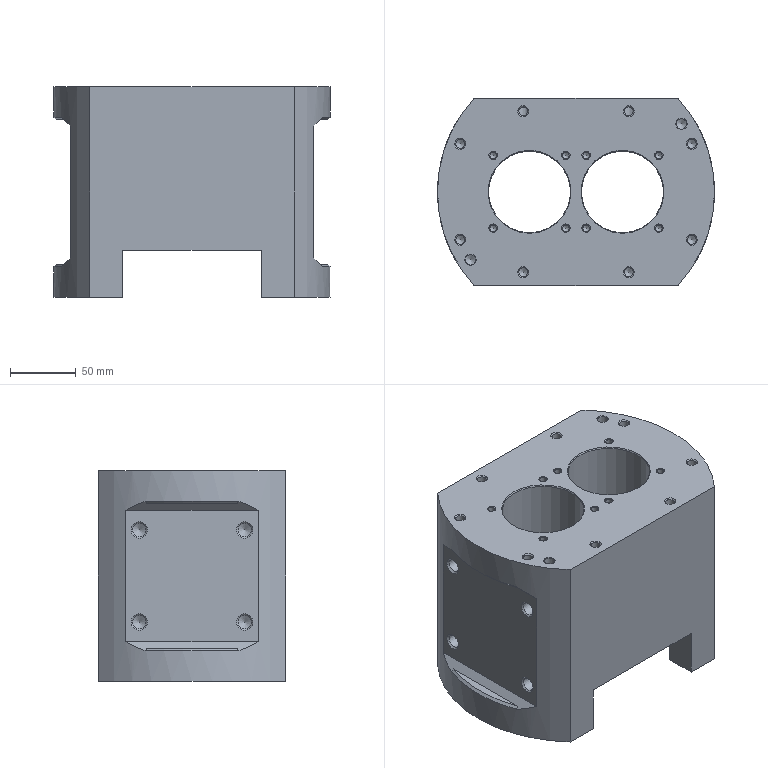NC program | NX | posted with a generic post | part box 210 x 142 x 160 mm
Lines 470 to 2090 of 4789, first 1533 of 1619 lines:
(ZLEVEL_PROFILE_COPY , TOOL : D10)
N932 T10 M6
N934 G54
N936 G17 G0 G90 X-54.432 Y32.868 B0. C0. S3500 M3
N938 G43 Z30. H10
N940 Z2.859
N942 G94 G1 Z-0.141 F1000.
N944 X-55.511 Y31.778
N946 G3 X-55.764 Y30.811 R1.
N948 G2 X-51.879 Y8.915 R121.943 F2200.
N950 X-53.503 Y-20.951 R111.959
N952 X-55.764 Y-30.811 R130.983
N954 G1 X-55.765 Y-30.984 Z-0.189
N956 X-55.768 Y-31.156 Z-0.236
N958 X-55.772 Y-31.328 Z-0.283
N960 G3 X-53.364 Y-20.951 R129.193
N962 G1 X-53.281 Y-20.505
N964 G3 X-51.988 Y11.59 R111.539
N966 X-55.772 Y31.328 R123.16
N968 G1 X-55.773 Y31.499 Z-0.33
N970 X-55.776 Y31.67 Z-0.377
N972 X-55.78 Y31.84 Z-0.424
N974 G2 X-52.279 Y15.115 R123.455
N976 X-52.684 Y-17.865 R110.827
N978 X-55.78 Y-31.84 R127.123
N980 G1 X-55.781 Y-32.011 Z-0.471
N982 X-55.783 Y-32.182 Z-0.519
N984 X-55.787 Y-32.352 Z-0.566
N986 G3 X-53.085 Y-20.951 R129.934
N988 X-51.753 Y12.035 R111.53
N990 X-55.788 Y32.352 R123.802
N992 G1 Y32.521 Z-0.613
N994 X-55.79 Y32.69 Z-0.66
N996 X-55.795 Y32.858 Z-0.707
N998 G2 X-51.882 Y14.264 R125.341
N1000 G1 X-51.666 Y12.481
N1002 G2 X-52.946 Y-20.951 R111.309
N1004 G1 X-53.031 Y-21.396
N1006 X-53.121 Y-21.842
N1008 G2 X-55.795 Y-32.858 R131.028
N1010 G1 X-55.797 Y-33.025 Z-0.754
N1012 X-55.8 Y-33.19 Z-0.801
N1014 X-55.804 Y-33.356 Z-0.849
N1016 G3 X-52.982 Y-21.842 R131.167
N1018 G1 X-52.893 Y-21.396
N1020 X-52.807 Y-20.951
N1022 G3 X-51.525 Y12.481 R111.179
N1024 G1 X-51.741 Y14.264
N1026 G3 X-55.804 Y33.356 R125.503
N1028 G1 X-55.807 Y33.521 Z-0.896
N1030 X-55.81 Y33.686 Z-0.943
N1032 X-55.814 Y33.851 Z-0.99
N1034 G2 X-51.657 Y14.71 R127.282
N1036 X-52.754 Y-21.396 R111.065
N1038 G1 X-52.843 Y-21.842
N1040 G2 X-55.814 Y-33.851 R132.662
N1042 G1 X-55.818 Y-34.012 Z-1.037
N1044 X-55.822 Y-34.173 Z-1.084
N1046 X-55.826 Y-34.334 Z-1.131
N1048 G3 X-52.705 Y-21.842 R131.086
N1050 G1 X-52.615 Y-21.396
N1052 G3 X-51.517 Y14.71 R110.891
N1054 X-55.826 Y34.334 R126.821
N1056 G1 X-55.831 Y34.495 Z-1.179
N1058 X-55.835 Y34.656 Z-1.226
N1060 X-55.841 Y34.816 Z-1.273
N1062 G2 X-51.377 Y14.71 R126.454
N1064 X-52.476 Y-21.396 R110.775
N1066 G1 X-52.566 Y-21.842
N1068 G2 X-55.841 Y-34.816 R130.126
N1070 G1 X-55.843 Y-34.978 Z-1.32
N1072 X-55.848 Y-35.139 Z-1.367
N1074 X-55.856 Y-35.298 Z-1.414
N1076 G3 X-52.427 Y-21.842 R130.376
N1078 G1 X-52.337 Y-21.396
N1080 G3 X-51.237 Y14.71 R110.658
N1082 X-55.856 Y35.298 R126.434
N1084 G1 Y35.459 Z-1.461
N1086 X-55.86 Y35.62 Z-1.508
N1088 X-55.871 Y35.778 Z-1.556
N1090 G2 X-51.097 Y14.71 R126.474
N1092 X-52.027 Y-20.505 R110.646
N1094 G1 X-52.111 Y-20.951
N1096 X-52.198 Y-21.396
N1098 X-52.288 Y-21.842
N1100 G2 X-55.871 Y-35.778 R131.039
N1102 G1 X-55.872 Y-35.939 Z-1.603
N1104 X-55.877 Y-36.098 Z-1.65
N1106 X-55.888 Y-36.255 Z-1.697
N1108 G3 X-51.496 Y-18.276 R129.399
N1110 X-51.349 Y17.385 R110.064
N1112 X-55.888 Y36.254 R129.287
N1114 G1 X-55.875 Y36.442 Z-1.768
N1116 X-55.868 Y36.628 Z-1.839
N1118 G2 X-51.281 Y17.83 R130.392
N1120 X-49.981 Y5.892 R114.798
N1122 X-49.9 Y3.02 R51.132
N1124 G1 Y-2.81
N1126 G2 X-50.037 Y-6.912 R61.409
N1128 X-53.454 Y-28.219 R117.255
N1130 G1 X-53.566 Y-28.655
N1132 G2 X-55.868 Y-36.629 R138.665
N1134 G1 X-55.801 Y-36.638 Z-1.909
N1136 X-55.709 Y-36.651 Z-1.98
N1138 X-55.636 Y-36.329
N1140 G3 X-53.174 Y-27.657 R143.814
N1142 X-50.01 Y-8.459 R118.727
N1144 X-49.9 Y-6.104 R34.261
N1146 G1 Y6.101
N1148 G3 X-50.011 Y8.469 R34.228
N1150 X-51.069 Y17.385 R117.375
N1152 X-55.289 Y35.215 R128.669
N1154 G1 X-55.653 Y36.391
N1156 G2 X-55.711 Y36.653 R1.62
N1158 G1 X-55.607 Y36.717 Z-2.051
N1160 X-55.524 Y36.779 Z-2.122
N1162 G3 X-55.381 Y35.942 R3.116
N1164 G1 X-55.292 Y35.661
N1166 G2 X-51.003 Y17.83 R129.054
N1168 X-49.949 Y9.361 R112.033
N1170 X-49.9 Y8.147 R16.61
N1172 G1 Y-8.249
N1174 G2 X-49.949 Y-9.361 R12.702
N1176 X-53.488 Y-29.42 R117.251
N1178 X-55.386 Y-35.966 R152.214
N1180 G3 X-55.513 Y-36.782 R2.768
N1182 G1 X-55.435 Y-36.945 Z-2.193
N1184 X-55.364 Y-37.108 Z-2.264
N1186 G2 X-55.295 Y-36.106 R10.195
N1188 G1 X-54.216 Y-32.54
N1190 X-54.089 Y-32.095
N1192 G3 X-50.017 Y-11.59 R120.931
N1194 X-49.9 Y-9.783 R18.135
N1196 G1 Y9.777
N1198 G3 X-50.017 Y11.59 R18.122
N1200 X-50.789 Y17.385 R128.233
N1202 X-55.298 Y36.106 R129.171
N1204 G2 X-55.365 Y37.107 R18.316
N1206 G1 X-55.283 Y37.269 Z-2.335
N1208 X-55.209 Y37.43 Z-2.407
N1210 X-55.183 Y36.329
N1212 X-55.162 Y36.106
N1214 G2 X-50.648 Y17.385 R129.227
N1216 X-49.966 Y12.339 R92.528
N1218 X-49.9 Y11.174 R11.539
N1220 G1 Y-11.172
N1222 G2 X-49.982 Y-12.481 R11.538
N1224 G1 X-50.015 Y-12.761
N1226 G2 X-53.142 Y-29.144 R118.996
N1228 X-55.159 Y-36.106 R155.69
N1230 G1 X-55.187 Y-36.329
N1232 X-55.208 Y-37.431
N1234 X-55.132 Y-37.584 Z-2.478
N1236 X-55.068 Y-37.738 Z-2.549
N1238 X-55.044 Y-36.329
N1240 X-55.023 Y-36.106
N1242 X-53.945 Y-32.54
N1244 X-53.815 Y-32.095
N1246 G3 X-50.053 Y-14.264 R122.421
N1248 G1 X-49.966 Y-13.53
N1250 G3 X-49.9 Y-12.411 R12.183
N1252 G1 Y12.41
N1254 G3 X-50.025 Y14.055 R14.641
N1256 X-51.051 Y20.505 R128.491
N1258 X-55.027 Y36.106 R132.287
N1260 G1 X-55.066 Y37.739
N1262 X-54.985 Y37.895 Z-2.62
N1264 X-54.918 Y38.051 Z-2.691
N1266 X-54.912 Y37.889
N1268 X-54.893 Y36.329
N1270 X-54.888 Y36.106
N1272 G2 X-50.911 Y20.505 R132.992
N1274 X-49.979 Y14.737 R101.49
N1276 X-49.9 Y13.534 R9.164
N1278 G1 Y-13.531
N1280 G2 X-49.976 Y-14.71 R9.171
N1282 X-53.809 Y-32.54 R121.679
N1284 G1 X-53.939 Y-32.986
N1286 X-54.887 Y-36.106
N1288 X-54.902 Y-36.329
N1290 X-54.913 Y-37.889
N1292 X-54.918 Y-38.05
N1294 X-54.844 Y-38.217 Z-2.762
N1296 X-54.775 Y-38.384 Z-2.833
N1298 X-54.773 Y-38.335
N1300 X-54.761 Y-36.329
N1302 X-54.749 Y-36.106
N1304 G3 X-53.042 Y-30.312 R181.888
N1306 X-49.985 Y-15.743 R119.356
N1308 X-49.9 Y-14.569 R8.156
N1310 G1 Y14.569
N1312 G3 X-49.985 Y15.748 R8.172
N1314 X-53.785 Y32.904 R120.132
N1316 G1 X-54.745 Y36.106
N1318 X-54.749 Y36.329
N1320 X-54.775 Y38.385
N1322 X-54.703 Y38.577 Z-2.904
N1324 X-54.633 Y38.768 Z-2.974
N1326 X-54.631 Y38.335
N1328 X-54.602 Y36.106
N1330 X-54.504 Y35.74
N1332 X-53.801 Y33.432
N1334 G2 X-50.089 Y17.385 R124.616
N1336 G1 X-50.019 Y16.939
N1338 G2 X-49.9 Y15.521 R9.442
N1340 G1 Y-15.524
N1342 G2 X-50.019 Y-16.939 R9.447
N1344 X-53.668 Y-32.986 R123.555
N1346 G1 X-53.801 Y-33.432
N1348 X-54.48 Y-35.661
N1350 X-54.611 Y-36.106
N1352 X-54.62 Y-36.329
N1354 X-54.632 Y-38.335
N1356 X-54.633 Y-38.768
N1358 X-54.562 Y-38.96 Z-3.045
N1360 X-54.492 Y-39.151 Z-3.116
N1362 X-54.491 Y-38.781
N1364 X-54.478 Y-36.329
N1366 X-54.473 Y-36.106
N1368 X-54.346 Y-35.661
N1370 X-53.666 Y-33.432
N1372 G3 X-50.027 Y-17.83 R123.17
N1374 X-49.9 Y-16.424 R8.031
N1376 G1 Y16.425
N1378 G3 X-50.007 Y17.714 R8.031
N1380 X-53.787 Y33.832 R123.645
N1382 G1 X-54.359 Y35.702
N1384 G2 X-54.459 Y36.106 R3.701
N1386 G1 X-54.492 Y39.152
N1388 X-54.421 Y39.339 Z-3.187
N1390 X-54.355 Y39.526 Z-3.257
N1392 X-54.315 Y36.106
N1394 G3 X-54.19 Y35.584 R4.242
N1396 G1 X-53.693 Y33.971
N1398 G2 X-50.03 Y18.661 R123.357
N1400 X-49.9 Y17.281 R8.995
N1402 G1 Y-17.278
N1404 G2 X-50.041 Y-18.722 R8.99
N1406 X-53.531 Y-33.432 R122.752
N1408 G1 X-54.211 Y-35.661
N1410 X-54.329 Y-36.106
N1412 X-54.335 Y-36.329
N1414 X-54.355 Y-39.526
N1416 X-54.28 Y-39.711 Z-3.328
N1418 X-54.214 Y-39.897 Z-3.399
N1420 X-54.197 Y-36.552
N1422 X-54.186 Y-36.106
N1424 G2 X-54.039 Y-35.54 R6.811
N1426 G1 X-53.621 Y-34.167
N1428 G3 X-50.054 Y-19.613 R124.955
N1430 X-49.9 Y-18.069 R8.702
N1432 G1 Y18.072
N1434 G3 X-50.013 Y19.375 R7.582
N1436 G1 X-50.132 Y20.059
N1438 G3 X-53.561 Y33.978 R126.794
N1440 G1 X-54.059 Y35.599
N1442 G2 X-54.171 Y36.106 R3.233
N1444 X-54.214 Y39.897 R175.513
N1446 G1 X-54.139 Y40.082 Z-3.469
N1448 X-54.071 Y40.268 Z-3.54
N1450 G3 X-54.01 Y35.884 R87.494
N1452 G2 X-50.043 Y20.308 R133.117
N1454 X-49.9 Y18.872 R7.449
N1456 G1 Y-18.868
N1458 G2 X-50.045 Y-20.342 R8.156
N1460 X-53.807 Y-35.215 R129.914
N1462 G1 X-54.01 Y-35.884
N1464 X-54.043 Y-36.106
N1466 X-54.056 Y-36.552
N1468 X-54.071 Y-40.268
N1470 X-53.997 Y-40.452 Z-3.611
N1472 X-53.93 Y-40.636 Z-3.682
N1474 X-53.918 Y-36.998
N1476 X-53.898 Y-36.045
N1478 X-53.899 Y-35.947
N1480 X-53.868 Y-35.854
N1482 X-53.673 Y-35.215
N1484 G3 X-50.031 Y-20.951 R126.56
N1486 X-49.9 Y-19.613 R8.173
N1488 G1 Y19.613
N1490 G3 X-50.031 Y20.951 R8.172
N1492 G1 X-50.478 Y23.179
N1494 G3 X-53.874 Y35.884 R137.422
N1496 G2 X-53.93 Y40.636 R126.824
N1498 G1 X-53.856 Y40.817 Z-3.752
N1500 X-53.786 Y40.997 Z-3.823
N1502 G3 X-53.738 Y35.884 R149.927
N1504 G2 X-51.271 Y27.191 R149.04
N1506 X-50.039 Y21.691 R108.525
N1508 X-49.9 Y20.31 R7.73
N1510 G1 Y-20.31
N1512 G2 X-50.04 Y-21.693 R7.73
N1514 G1 X-50.157 Y-22.288
N1516 G2 X-53.701 Y-35.742 R131.324
N1518 G3 X-53.755 Y-36.065 R1.144
N1520 G1 X-53.777 Y-36.998
N1522 X-53.786 Y-40.997
N1524 X-53.715 Y-41.175 Z-3.894
N1526 X-53.647 Y-41.353 Z-3.964
N1528 X-53.627 Y-36.552
N1530 X-53.606 Y-35.884
N1532 X-52.927 Y-33.664
N1534 G3 X-50.082 Y-22.614 R127.066
N1536 X-49.9 Y-21.023 R8.589
N1538 G1 Y21.024
N1540 G3 X-50.107 Y22.734 R8.344
N1542 X-53.602 Y35.884 R137.68
N1544 G2 X-53.647 Y41.353 R180.835
N1546 G1 X-53.573 Y41.531 Z-4.035
N1548 X-53.507 Y41.709 Z-4.106
N1550 X-53.488 Y36.998
N1552 X-53.464 Y35.884
N1554 G2 X-51.982 Y30.899 R200.497
N1556 X-50.045 Y23.08 R121.054
N1558 X-49.9 Y21.692 R6.607
N1560 G1 Y-21.693
N1562 G2 X-50.066 Y-23.179 R6.607
N1564 X-53.271 Y-35.215 R128.592
N1566 G1 X-53.465 Y-35.884
N1568 X-53.494 Y-36.998
N1570 X-53.507 Y-41.709
N1572 X-53.432 Y-41.886 Z-4.177
N1574 X-53.365 Y-42.062 Z-4.247
N1576 X-53.352 Y-36.998
N1578 X-53.325 Y-35.884
N1580 G2 X-53.153 Y-35.264 R8.237
N1582 G3 X-50.089 Y-23.898 R126.07
N1584 X-49.9 Y-22.343 R7.321
N1586 G1 Y22.34
N1588 G3 X-50.089 Y23.898 R7.319
N1590 X-52.316 Y32.54 R122.932
N1592 G1 X-52.449 Y32.986
N1594 X-53.268 Y35.661
N1596 X-53.326 Y35.884
N1598 X-53.349 Y36.998
N1600 X-53.365 Y42.062
N1602 X-53.291 Y42.236 Z-4.318
N1604 X-53.222 Y42.41 Z-4.389
N1606 X-53.209 Y36.998
N1608 X-53.179 Y35.831
N1610 G2 X-51.062 Y28.529 R168.448
N1612 X-50.065 Y24.405 R94.608
N1614 X-49.9 Y22.939 R7.176
N1616 G1 Y-22.939
N1618 G2 X-50.089 Y-24.514 R7.176
N1620 X-53.003 Y-35.215 R126.158
N1622 G1 X-53.179 Y-35.833
N1624 X-53.185 Y-35.884
N1626 X-53.211 Y-36.998
N1628 X-53.222 Y-42.41
N1630 X-53.149 Y-42.581 Z-4.459
N1632 X-53.079 Y-42.753 Z-4.53
N1634 X-53.07 Y-36.998
N1636 X-53.049 Y-36.018
N1638 G2 X-52.964 Y-35.513 R1.77
N1640 G3 X-50.107 Y-25.216 R130.635
N1642 X-49.9 Y-23.58 R7.925
N1644 G1 Y23.583
N1646 G3 X-50.109 Y25.229 R7.96
N1648 X-52.889 Y35.302 R136.594
N1650 G2 X-53.052 Y35.884 R8.691
N1652 G1 X-53.063 Y36.552
N1654 X-53.079 Y42.753
N1656 X-53.008 Y42.924 Z-4.601
N1658 X-52.943 Y43.095 Z-4.672
N1660 X-52.937 Y42.793
N1662 X-52.93 Y36.998
N1664 X-52.915 Y35.884
N1666 G3 X-52.785 Y35.398 R5.311
N1668 G2 X-50.12 Y25.854 R137.331
N1670 G1 X-50.089 Y25.724
N1672 G2 X-49.9 Y24.175 R6.811
N1674 G1 Y-24.175
N1676 G2 X-50.089 Y-25.724 R6.811
N1678 G1 X-50.12 Y-25.854
N1680 G2 X-52.871 Y-35.661 R136.202
N1682 G3 X-52.911 Y-35.968 R1.414
N1684 G1 X-52.929 Y-36.998
N1686 X-52.937 Y-42.793
N1688 X-52.943 Y-43.095
N1690 X-52.866 Y-43.266 Z-4.742
N1692 X-52.8 Y-43.436 Z-4.813
N1694 X-52.789 Y-36.998
N1696 X-52.775 Y-35.972
N1698 G2 X-52.738 Y-35.662 R1.5
N1700 G3 X-50.089 Y-26.279 R133.327
N1702 X-49.9 Y-24.757 R6.307
N1704 G1 Y24.754
N1706 G3 X-50.08 Y26.241 R6.308
N1708 X-52.7 Y35.534 R137.177
N1710 G2 X-52.788 Y36.093 R1.844
N1712 G1 X-52.8 Y43.436
N1714 X-52.725 Y43.603 Z-4.884
N1716 X-52.658 Y43.771 Z-4.954
N1718 X-52.649 Y36.552
N1720 X-52.642 Y35.989
N1722 G3 X-52.572 Y35.563 R1.449
N1724 G2 X-50.069 Y26.746 R130.164
N1726 X-49.9 Y25.32 R6.312
N1728 G1 Y-25.32
N1730 G2 X-50.069 Y-26.746 R6.313
N1732 X-52.604 Y-35.661 R130.762
N1734 G3 X-52.641 Y-36.123 R3.13
N1736 G1 X-52.652 Y-37.889
N1738 X-52.654 Y-43.684
N1740 X-52.658 Y-43.771
N1742 X-52.584 Y-43.935 Z-5.025
N1744 X-52.514 Y-44.1 Z-5.096
N1746 X-52.511 Y-37.889
N1748 X-52.503 Y-36.181
N1750 G2 X-52.47 Y-35.661 R4.446
N1752 G3 X-50.089 Y-27.376 R132.107
N1754 X-49.9 Y-25.854 R6.364
N1756 G1 Y25.854
N1758 G3 X-50.089 Y27.376 R6.365
N1760 X-52.433 Y35.542 R129.965
N1762 G2 X-52.504 Y35.986 R1.482
N1764 G1 X-52.508 Y36.552
N1766 X-52.514 Y44.1
N1768 X-52.442 Y44.264 Z-5.166
N1770 X-52.376 Y44.429 Z-5.237
N1772 X-52.371 Y44.13
N1774 X-52.37 Y37.444
N1776 X-52.366 Y35.884
N1778 G3 X-52.266 Y35.44 R2.54
N1780 G2 X-50.129 Y28.083 R137.295
N1782 X-49.9 Y26.413 R6.52
N1784 G1 Y-26.414
N1786 G2 X-50.129 Y-28.083 R6.52
N1788 X-52.336 Y-35.661 R140.023
N1790 G1 X-52.366 Y-36.552
N1792 X-52.37 Y-37.889
N1794 X-52.371 Y-44.13
N1796 X-52.376 Y-44.429
N1798 X-52.301 Y-44.593 Z-5.308
N1800 X-52.234 Y-44.757 Z-5.379
N1802 X-52.226 Y-36.998
N1804 X-52.202 Y-35.661
N1806 G3 X-50.107 Y-28.529 R144.816
N1808 X-49.9 Y-26.942 R6.264
N1810 G1 Y26.941
N1812 G3 X-50.089 Y28.457 R6.229
N1814 X-52.172 Y35.56 R139.356
N1816 G2 X-52.227 Y35.911 R1.151
N1818 G1 X-52.229 Y37.444
N1820 X-52.23 Y44.576
N1822 X-52.234 Y44.758
N1824 X-52.159 Y44.92 Z-5.449
N1826 X-52.091 Y45.083 Z-5.52
N1828 X-52.089 Y45.022
N1830 X-52.088 Y37.444
N1832 X-52.085 Y35.742
N1834 G2 X-50.094 Y28.974 R157.101
N1836 X-49.9 Y27.459 R6.092
N1838 G1 Y-27.458
N1840 G2 X-50.089 Y-28.955 R6.103
N1842 X-52.067 Y-35.661 R139.741
N1844 G1 X-52.085 Y-36.552
N1846 X-52.091 Y-45.083
N1848 X-52.018 Y-45.242 Z-5.591
N1850 X-51.949 Y-45.4 Z-5.661
N1852 X-51.942 Y-36.106
N1854 X-51.932 Y-35.661
N1856 G3 X-50.089 Y-29.449 R138.342
N1858 X-49.9 Y-27.967 R6.104
N1860 G1 Y27.967
N1862 G3 X-50.089 Y29.449 R6.104
N1864 X-51.936 Y35.661 R130.385
N1866 G1 X-51.945 Y35.771
N1868 X-51.949 Y45.4
N1870 X-51.876 Y45.559 Z-5.732
N1872 X-51.809 Y45.717 Z-5.803
N1874 X-51.806 Y45.467
N1876 X-51.805 Y36.552
N1878 X-51.803 Y35.661
N1880 G2 X-50.108 Y30.01 R126.296
N1882 X-49.9 Y28.468 R5.822
N1884 G1 Y-28.465
N1886 G2 X-50.111 Y-30.022 R5.844
N1888 X-51.795 Y-35.661 R144.119
N1890 G1 X-51.803 Y-36.106
N1892 X-51.806 Y-45.467
N1894 X-51.809 Y-45.717
N1896 X-51.735 Y-45.876 Z-5.874
N1898 X-51.67 Y-46.034 Z-5.944
N1900 X-51.658 Y-35.661
N1902 G3 X-50.177 Y-30.757 R207.506
N1904 X-49.9 Y-28.951 R6.463
N1906 G1 Y28.952
N1908 G3 X-50.177 Y30.757 R6.464
N1910 X-51.664 Y35.661 R169.662
N1912 G1 Y45.913
N1914 X-51.67 Y46.034
N1916 X-51.594 Y46.193 Z-6.015
N1918 X-51.523 Y46.352 Z-6.086
N1920 X-51.522 Y35.661
N1922 G2 X-50.166 Y31.203 R440.41
N1924 X-49.9 Y29.42 R6.342
N1926 G1 Y-29.42
N1928 G2 X-50.166 Y-31.203 R6.342
N1930 G1 X-50.969 Y-33.878
N1932 X-51.491 Y-35.555
N1934 X-51.52 Y-35.661
N1936 X-51.522 Y-36.106
N1938 X-51.523 Y-46.352
N1940 X-51.452 Y-46.505 Z-6.156
N1942 X-51.383 Y-46.658 Z-6.227
N1944 X-51.381 Y-46.359
N1946 Y-35.6
N1948 G3 X-50.165 Y-31.649 R143.282
N1950 X-49.9 Y-29.901 R6.098
N1952 G1 Y29.902
N1954 G3 X-50.165 Y31.649 R6.098
N1956 X-51.381 Y35.6 R143.247
N1958 G1 Y46.359
N1960 X-51.383 Y46.658
N1962 X-51.311 Y46.811 Z-6.298
N1964 X-51.246 Y46.963 Z-6.369
N1966 X-51.24 Y46.805
N1968 Y35.575
N1970 G2 X-50.164 Y32.095 R124.433
N1972 X-49.9 Y30.366 R6.1
N1974 G1 Y-30.367
N1976 G2 X-50.164 Y-32.095 R6.101
N1978 X-51.24 Y-35.575 R124.395
N1980 G1 Y-46.805
N1982 X-51.246 Y-46.963
N1984 X-51.169 Y-47.116 Z-6.439
N1986 X-51.1 Y-47.269 Z-6.51
N1988 X-51.099 Y-36.586
N1990 Y-35.55
N1992 G3 X-50.163 Y-32.54 R110.245
N1994 X-49.9 Y-30.819 R6.103
N1996 G1 Y30.821
N1998 G3 X-50.163 Y32.54 R6.104
N2000 X-51.099 Y35.55 R110.245
N2002 G1 Y36.587
N2004 X-51.1 Y47.269
N2006 X-51.028 Y47.422 Z-6.581
N2008 X-50.958 Y47.575 Z-6.651
N2010 X-50.957 Y36.965
N2012 Y35.525
N2014 X-50.296 Y33.432
N2016 X-50.162 Y32.986
N2018 G2 X-49.9 Y31.268 R6.106
N2020 G1 Y-31.269
N2022 G2 X-50.162 Y-32.986 R6.107
N2024 G1 X-50.296 Y-33.432
N2026 X-50.957 Y-35.525
N2028 Y-47.25
N2030 X-50.958 Y-47.575
N2032 X-50.886 Y-47.725 Z-6.722
N2034 X-50.821 Y-47.875 Z-6.793
N2036 X-50.816 Y-47.696
N2038 Y-35.5
N2040 X-50.161 Y-33.432
N2042 G3 X-49.9 Y-31.709 R6.108
N2044 G1 Y31.712
N2046 G3 X-50.161 Y33.432 R6.109
N2048 G1 X-50.816 Y35.5
N2050 Y47.696
N2052 X-50.821 Y47.875
N2054 X-50.745 Y48.023 Z-6.864
N2056 X-50.676 Y48.171 Z-6.934
N2058 X-50.674 Y37.444
N2060 Y35.465
N2062 X-50.183 Y33.944
N2064 G2 X-49.9 Y32.147 R5.851
N2066 G1 Y-32.147
N2068 G2 X-50.183 Y-33.944 R5.851
N2070 G1 X-50.674 Y-35.465
N2072 Y-37.444
N2074 X-50.676 Y-48.171
N2076 X-50.604 Y-48.319 Z-7.005
N2078 X-50.534 Y-48.466 Z-7.076
N2080 X-50.533 Y-38.074
N2082 X-50.532 Y-35.44
N2084 X-50.172 Y-34.323
N2086 G3 X-49.9 Y-32.572 R5.963
N2088 G1 Y32.573
N2090 G3 X-50.172 Y34.323 R5.963
N2092 G1 X-50.532 Y35.44
N2094 X-50.533 Y38.074
N2096 X-50.534 Y48.466
N2098 X-50.462 Y48.614 Z-7.146
N2100 X-50.397 Y48.761 Z-7.217
N2102 X-50.391 Y48.588
N2104 Y35.416
N2106 X-50.183 Y34.769
N2108 G2 X-49.9 Y32.986 R5.931
N2110 G1 Y-32.986
N2112 G2 X-50.183 Y-34.769 R5.931
N2114 G1 X-50.391 Y-35.416
N2116 Y-48.588
N2118 X-50.397 Y-48.761
N2120 X-50.321 Y-48.909 Z-7.288
N2122 X-50.251 Y-49.056 Z-7.359
N2124 X-50.25 Y-38.781
N2126 Y-35.394
N2128 G3 X-49.9 Y-33.41 R6.093
N2130 G1 Y33.41
N2132 G3 X-50.25 Y35.394 R6.093
N2134 G1 Y38.781
N2136 X-50.251 Y49.056
N2138 X-50.179 Y49.2 Z-7.429
N2140 X-50.111 Y49.343 Z-7.5
N2142 X-50.109 Y38.781
N2144 Y35.361
N2146 G2 X-49.9 Y33.823 R6.101
N2148 G1 Y-33.821
N2150 G2 X-50.109 Y-35.361 R6.101
N2152 G1 Y-38.781
N2154 X-50.111 Y-49.343
N2156 X-50.038 Y-49.486 Z-7.571
N2158 X-49.972 Y-49.629 Z-7.641
N2160 X-49.967 Y-49.479
N2162 Y-35.181
N2164 G3 X-49.9 Y-34.225 R11.45
N2166 G1 Y34.226
N2168 G3 X-49.967 Y35.181 R11.463
N2170 G1 Y49.479
N2172 X-49.972 Y49.629
N2174 X-49.897 Y49.771 Z-7.712
N2176 X-49.826 Y49.914 Z-7.783
N2178 Y39.672
N2180 Y-39.672
N2182 Y-49.914
N2184 X-49.755 Y-50.056 Z-7.853
N2186 X-49.688 Y-50.199 Z-7.924
N2188 X-49.684 Y-49.925
N2190 Y49.925
N2192 X-49.688 Y50.199
N2194 X-49.614 Y50.34 Z-7.995
N2196 X-49.547 Y50.48 Z-8.066
N2198 X-49.543 Y50.371
N2200 X-49.542 Y40.528
N2202 X-49.543 Y40.118
N2204 Y-40.118
N2206 X-49.542 Y-40.528
N2208 X-49.543 Y-50.371
N2210 X-49.547 Y-50.48
N2212 X-49.472 Y-50.619 Z-8.136
N2214 X-49.404 Y-50.758 Z-8.207
N2216 X-49.402 Y-50.371
N2218 Y50.371
N2220 X-49.404 Y50.758
N2222 X-49.331 Y50.896 Z-8.278
N2224 X-49.264 Y51.034 Z-8.348
N2226 X-49.26 Y50.816
N2228 Y-50.816
N2230 X-49.264 Y-51.034
N2232 X-49.189 Y-51.172 Z-8.419
N2234 X-49.121 Y-51.31 Z-8.49
N2236 X-49.119 Y-41.456
N2238 Y41.456
N2240 X-49.121 Y51.31
N2242 X-49.048 Y51.447 Z-8.561
N2244 X-48.982 Y51.585 Z-8.631
N2246 X-48.977 Y51.262
N2248 X-48.976 Y41.855
N2250 X-48.977 Y41.456
N2252 Y-41.456
N2254 X-48.976 Y-41.855
N2256 X-48.977 Y-51.262
N2258 X-48.982 Y-51.585
N2260 X-48.907 Y-51.721 Z-8.702
N2262 X-48.84 Y-51.858 Z-8.773
N2264 X-48.836 Y-51.708
N2266 Y51.708
N2268 X-48.84 Y51.858
N2270 X-48.765 Y51.992 Z-8.843
N2272 X-48.695 Y52.126 Z-8.914
N2274 X-48.694 Y42.347
N2276 Y-42.347
N2278 X-48.695 Y-52.126
N2280 X-48.624 Y-52.259 Z-8.985
N2282 X-48.559 Y-52.392 Z-9.056
N2284 X-48.553 Y-52.154
N2286 Y52.154
N2288 X-48.559 Y52.392
N2290 X-48.482 Y52.526 Z-9.126
N2292 X-48.414 Y52.659 Z-9.197
N2294 X-48.412 Y42.793
N2296 Y-42.793
N2298 X-48.414 Y-52.659
N2300 X-48.341 Y-52.792 Z-9.268
N2302 X-48.272 Y-52.925 Z-9.338
N2304 X-48.27 Y-52.599
N2306 Y52.599
N2308 X-48.272 Y52.925
N2310 X-48.199 Y53.057 Z-9.409
N2312 X-48.134 Y53.19 Z-9.48
N2314 X-48.129 Y53.045
N2316 Y-53.045
N2318 X-48.134 Y-53.19
N2320 X-48.058 Y-53.322 Z-9.551
N2322 X-47.989 Y-53.453 Z-9.621
N2324 X-47.987 Y-43.684
N2326 Y43.684
N2328 X-47.989 Y53.453
N2330 X-47.917 Y53.585 Z-9.692
N2332 X-47.849 Y53.716 Z-9.763
N2334 X-47.846 Y53.491
N2336 Y-53.491
N2338 X-47.849 Y-53.716
N2340 X-47.775 Y-53.847 Z-9.833
N2342 X-47.707 Y-53.978 Z-9.904
N2344 X-47.704 Y-53.937
N2346 Y53.937
N2348 X-47.707 Y53.978
N2350 X-47.634 Y54.109 Z-9.975
N2352 X-47.569 Y54.241 Z-10.046
N2354 X-47.563 Y53.937
N2356 Y-53.937
N2358 X-47.569 Y-54.241
N2360 X-47.492 Y-54.372 Z-10.116
N2362 X-47.425 Y-54.503 Z-10.187
N2364 X-47.422 Y-54.383
N2366 Y54.383
N2368 X-47.425 Y54.503
N2370 X-47.351 Y54.634 Z-10.258
N2372 X-47.282 Y54.765 Z-10.328
N2374 X-47.28 Y45.467
N2376 Y-45.467
N2378 X-47.282 Y-54.766
N2380 X-47.21 Y-54.897 Z-10.399
N2382 X-47.143 Y-55.028 Z-10.47
N2384 X-47.139 Y-54.828
N2386 Y54.828
N2388 X-47.143 Y55.028
N2390 X-47.068 Y55.159 Z-10.54
N2392 X-46.998 Y55.29 Z-10.611
N2394 X-46.997 Y46.143
N2396 Y-46.142
N2398 X-46.998 Y-55.29
N2400 X-46.927 Y-55.422 Z-10.682
N2402 X-46.86 Y-55.553 Z-10.753
N2404 X-46.856 Y-55.274
N2406 Y55.274
N2408 X-46.86 Y55.552
N2410 X-46.785 Y55.684 Z-10.823
N2412 X-46.718 Y55.815 Z-10.894
N2414 X-46.715 Y55.72
N2416 Y-55.72
N2418 X-46.718 Y-55.815
N2420 X-46.644 Y-55.946 Z-10.965
N2422 X-46.574 Y-56.077 Z-11.035
N2424 X-46.573 Y-46.805
N2426 Y46.805
N2428 X-46.574 Y56.077
N2430 X-46.502 Y56.209 Z-11.106
N2432 X-46.436 Y56.34 Z-11.177
N2434 X-46.432 Y56.166
N2436 Y-56.166
N2438 X-46.436 Y-56.34
N2440 X-46.361 Y-56.471 Z-11.248
N2442 X-46.291 Y-56.602 Z-11.318
N2444 X-46.29 Y-47.25
N2446 Y47.25
N2448 X-46.291 Y56.602
N2450 X-46.22 Y56.733 Z-11.389
N2452 X-46.152 Y56.865 Z-11.46
N2454 X-46.149 Y56.611
N2456 Y-56.611
N2458 X-46.152 Y-56.865
N2460 X-46.078 Y-56.996 Z-11.53
N2462 X-46.01 Y-57.127 Z-11.601
N2464 X-46.007 Y-57.057
N2466 Y57.057
N2468 X-46.01 Y57.127
N2470 X-45.937 Y57.258 Z-11.672
N2472 X-45.87 Y57.389 Z-11.743
N2474 X-45.866 Y57.057
N2476 Y-57.057
N2478 X-45.87 Y-57.389
N2480 X-45.795 Y-57.521 Z-11.813
N2482 X-45.728 Y-57.652 Z-11.884
N2484 X-45.725 Y-57.503
N2486 Y57.503
N2488 X-45.728 Y57.652
N2490 X-45.654 Y57.783 Z-11.955
N2492 X-45.584 Y57.914 Z-12.025
N2494 X-45.583 Y48.588
N2496 Y-48.588
N2498 X-45.584 Y-57.914
N2500 X-45.512 Y-58.045 Z-12.096
N2502 X-45.448 Y-58.176 Z-12.167
N2504 X-45.442 Y-57.949
N2506 Y57.949
N2508 X-45.448 Y58.176
N2510 X-45.381 Y58.288 Z-12.227
N2512 X-45.321 Y58.401 Z-12.288
N2514 Y49.033
N2516 Y-49.033
N2518 Y-58.401
N2520 X-45.261 Y-58.513 Z-12.348
N2522 X-45.203 Y-58.625 Z-12.408
N2524 X-45.2 Y-58.394
N2526 Y58.394
N2528 X-45.203 Y58.625
N2530 X-45.14 Y58.737 Z-12.469
N2532 X-45.08 Y58.849 Z-12.529
N2534 X-45.079 Y49.872
N2536 Y-49.872
N2538 X-45.08 Y-58.849
N2540 X-45.019 Y-58.959 Z-12.59
N2542 X-44.968 Y-59.068 Z-12.65
N2544 X-44.961 Y-58.84
N2546 Y58.84
N2548 X-44.968 Y59.068
N2550 G2 X-44.495 Y59.949 R1.
N2552 G1 X-43.17 Y60.769
N2554 Z-9.65
N2556 G0 Z30.
N2558 X54.432 Y-32.868
N2560 Z2.859
N2562 G1 Z-0.141 F1000.
N2564 X55.511 Y-31.778
N2566 G3 X55.764 Y-30.811 R1.
N2568 G2 X51.879 Y-8.915 R121.944 F2200.
N2570 X53.503 Y20.951 R111.959
N2572 X55.764 Y30.81 R130.986
N2574 G1 X55.765 Y30.984 Z-0.189
N2576 X55.768 Y31.156 Z-0.236
N2578 X55.772 Y31.328 Z-0.283
N2580 G3 X53.364 Y20.951 R129.193
N2582 G1 X53.281 Y20.505
N2584 G3 X51.988 Y-11.59 R111.539
N2586 X55.772 Y-31.328 R123.159
N2588 G1 X55.773 Y-31.499 Z-0.33
N2590 X55.776 Y-31.67 Z-0.377
N2592 X55.78 Y-31.84 Z-0.424
N2594 G2 X52.278 Y-15.109 R123.455
N2596 X52.684 Y17.86 R110.823
N2598 X55.78 Y31.84 R127.123
N2600 G1 X55.781 Y32.011 Z-0.471
N2602 X55.783 Y32.182 Z-0.519
N2604 X55.788 Y32.352 Z-0.566
N2606 G3 X53.085 Y20.951 R129.934
N2608 X51.753 Y-12.035 R111.53
N2610 X55.788 Y-32.352 R123.802
N2612 G1 Y-32.521 Z-0.613
N2614 X55.79 Y-32.69 Z-0.66
N2616 X55.795 Y-32.858 Z-0.707
N2618 G2 X51.882 Y-14.264 R125.341
N2620 G1 X51.666 Y-12.481
N2622 G2 X52.946 Y20.951 R111.309
N2624 G1 X53.031 Y21.396
N2626 X53.121 Y21.842
N2628 G2 X55.795 Y32.859 R130.426
N2630 G1 X55.797 Y33.025 Z-0.754
N2632 X55.8 Y33.19 Z-0.801
N2634 X55.804 Y33.356 Z-0.849
N2636 G3 X52.982 Y21.842 R131.167
N2638 G1 X52.893 Y21.396
N2640 X52.807 Y20.951
N2642 G3 X51.525 Y-12.481 R111.179
N2644 G1 X51.741 Y-14.264
N2646 G3 X55.804 Y-33.356 R125.503
N2648 G1 X55.807 Y-33.521 Z-0.896
N2650 X55.81 Y-33.686 Z-0.943
N2652 X55.814 Y-33.851 Z-0.99
N2654 G2 X51.657 Y-14.71 R127.282
N2656 X52.754 Y21.396 R111.05
N2658 G1 X52.843 Y21.842
N2660 G2 X55.814 Y33.85 R132.754
N2662 G1 X55.818 Y34.012 Z-1.037
N2664 X55.822 Y34.173 Z-1.084
N2666 X55.826 Y34.334 Z-1.131
N2668 G3 X52.705 Y21.842 R131.086
N2670 G1 X52.615 Y21.396
N2672 G3 X51.517 Y-14.71 R110.891
N2674 X55.826 Y-34.334 R126.821
N2676 G1 X55.831 Y-34.495 Z-1.179
N2678 X55.835 Y-34.656 Z-1.226
N2680 X55.841 Y-34.816 Z-1.273
N2682 G2 X51.377 Y-14.71 R126.455
N2684 X52.476 Y21.396 R110.775
N2686 G1 X52.566 Y21.842
N2688 G2 X55.841 Y34.816 R130.13
N2690 G1 X55.843 Y34.978 Z-1.32
N2692 X55.848 Y35.138 Z-1.367
N2694 X55.856 Y35.298 Z-1.414
N2696 G3 X52.427 Y21.842 R130.358
N2698 G1 X52.337 Y21.396
N2700 G3 X51.237 Y-14.71 R110.658
N2702 X55.856 Y-35.298 R126.432
N2704 G1 Y-35.459 Z-1.461
N2706 X55.86 Y-35.62 Z-1.508
N2708 X55.871 Y-35.778 Z-1.556
N2710 G2 X51.097 Y-14.71 R126.475
N2712 X52.027 Y20.505 R110.646
N2714 G1 X52.111 Y20.951
N2716 X52.198 Y21.396
N2718 X52.296 Y21.883
N2720 G2 X55.871 Y35.779 R131.022
N2722 G1 X55.872 Y35.939 Z-1.603
N2724 X55.877 Y36.098 Z-1.65
N2726 X55.888 Y36.255 Z-1.697
N2728 G3 X51.496 Y18.276 R129.4
N2730 X51.349 Y-17.385 R110.064
N2732 X55.888 Y-36.254 R129.287
N2734 G1 X55.875 Y-36.442 Z-1.768
N2736 X55.868 Y-36.628 Z-1.839
N2738 G2 X51.281 Y-17.83 R130.392
N2740 X49.981 Y-5.892 R114.798
N2742 X49.9 Y-3.02 R51.132
N2744 G1 Y2.81
N2746 G2 X50.037 Y6.912 R61.409
N2748 X53.454 Y28.219 R117.255
N2750 G1 X53.569 Y28.667
N2752 G2 X55.868 Y36.629 R138.248
N2754 G1 X55.801 Y36.638 Z-1.909
N2756 X55.709 Y36.651 Z-1.98
N2758 X55.636 Y36.329
N2760 G3 X53.174 Y27.657 R143.814
N2762 X50.01 Y8.459 R118.727
N2764 X49.9 Y6.104 R34.261
N2766 G1 Y-6.101
N2768 G3 X50.011 Y-8.469 R34.228
N2770 X51.069 Y-17.385 R117.375
N2772 X55.289 Y-35.215 R128.669
N2774 G1 X55.653 Y-36.391
N2776 G2 X55.711 Y-36.653 R1.62
N2778 G1 X55.607 Y-36.717 Z-2.051
N2780 X55.524 Y-36.779 Z-2.122
N2782 G3 X55.381 Y-35.942 R3.116
N2784 G1 X55.292 Y-35.661
N2786 G2 X51.003 Y-17.83 R129.054
N2788 X49.958 Y-9.478 R103.719
N2790 X49.9 Y-8.147 R16.61
N2792 G1 Y8.246
N2794 G2 X49.95 Y9.37 R12.771
N2796 X53.111 Y27.961 R117.548
N2798 X55.386 Y35.966 R147.96
N2800 G3 X55.513 Y36.782 R2.761
N2802 G1 X55.435 Y36.945 Z-2.193
N2804 X55.364 Y37.108 Z-2.264
N2806 G2 X55.295 Y36.106 R10.196
N2808 G1 X54.216 Y32.54
N2810 X54.089 Y32.095
N2812 G3 X50.017 Y11.59 R120.931
N2814 X49.9 Y9.783 R18.135
N2816 G1 Y-9.777
N2818 G3 X50.017 Y-11.59 R18.122
N2820 X50.789 Y-17.385 R125.204
N2822 X55.298 Y-36.106 R129.171
N2824 G2 X55.365 Y-37.107 R18.316
N2826 G1 X55.283 Y-37.269 Z-2.335
N2828 X55.209 Y-37.43 Z-2.407
N2830 X55.183 Y-36.329
N2832 X55.162 Y-36.106
N2834 G2 X50.648 Y-17.385 R129.227
N2836 X49.966 Y-12.339 R92.528
N2838 X49.9 Y-11.174 R11.539
N2840 G1 Y11.172
N2842 G2 X49.982 Y12.481 R11.538
N2844 G1 X50.015 Y12.761
N2846 G2 X53.142 Y29.144 R118.996
N2848 X55.159 Y36.106 R155.69
N2850 G1 X55.187 Y36.329
N2852 X55.208 Y37.431
N2854 X55.132 Y37.584 Z-2.478
N2856 X55.068 Y37.738 Z-2.549
N2858 X55.044 Y36.329
N2860 X55.023 Y36.106
N2862 X53.945 Y32.54
N2864 X53.815 Y32.095
N2866 G3 X50.053 Y14.264 R122.421
N2868 G1 X49.966 Y13.53
N2870 G3 X49.9 Y12.411 R12.183
N2872 G1 Y-12.41
N2874 G3 X50.025 Y-14.055 R14.641
N2876 X51.051 Y-20.505 R128.491
N2878 X55.027 Y-36.106 R132.287
N2880 G1 X55.066 Y-37.739
N2882 X54.985 Y-37.895 Z-2.62
N2884 X54.918 Y-38.051 Z-2.691
N2886 X54.912 Y-37.889
N2888 X54.893 Y-36.329
N2890 X54.888 Y-36.106
N2892 G2 X50.911 Y-20.505 R132.992
N2894 X49.979 Y-14.737 R101.49
N2896 X49.9 Y-13.534 R9.164
N2898 G1 Y13.531
N2900 G2 X49.976 Y14.71 R9.171
N2902 X53.809 Y32.54 R121.679
N2904 G1 X53.939 Y32.986
N2906 X54.887 Y36.106
N2908 X54.902 Y36.329
N2910 X54.913 Y37.889
N2912 X54.918 Y38.05
N2914 X54.844 Y38.217 Z-2.762
N2916 X54.775 Y38.384 Z-2.833
N2918 X54.773 Y38.335
N2920 X54.761 Y36.329
N2922 X54.749 Y36.106
N2924 G3 X53.042 Y30.312 R181.888
N2926 X49.985 Y15.743 R119.348
N2928 X49.9 Y14.569 R8.156
N2930 G1 Y-14.569
N2932 G3 X49.985 Y-15.748 R8.172
N2934 X53.785 Y-32.904 R120.132
N2936 G1 X54.745 Y-36.106
N2938 X54.749 Y-36.329
N2940 X54.775 Y-38.385
N2942 X54.703 Y-38.576 Z-2.904
N2944 X54.633 Y-38.768 Z-2.974
N2946 X54.631 Y-38.335
N2948 X54.602 Y-36.106
N2950 X54.504 Y-35.74
N2952 X53.801 Y-33.432
N2954 G2 X50.089 Y-17.385 R124.616
N2956 G1 X50.019 Y-16.939
N2958 G2 X49.9 Y-15.521 R9.442
N2960 G1 Y15.524
N2962 G2 X50.019 Y16.939 R9.447
N2964 X53.668 Y32.986 R123.555
N2966 G1 X53.801 Y33.432
N2968 X54.48 Y35.661
N2970 X54.611 Y36.106
N2972 X54.62 Y36.329
N2974 X54.632 Y38.335
N2976 X54.633 Y38.768
N2978 X54.562 Y38.96 Z-3.045
N2980 X54.492 Y39.152 Z-3.116
N2982 X54.491 Y38.781
N2984 X54.478 Y36.329
N2986 X54.473 Y36.106
N2988 X54.346 Y35.661
N2990 X53.666 Y33.432
N2992 G3 X50.027 Y17.83 R123.169
N2994 X49.9 Y16.424 R8.031
N2996 G1 Y-16.425
N2998 G3 X50.007 Y-17.714 R8.031
N3000 X53.787 Y-33.832 R123.645
N3002 G1 X54.355 Y-35.688
N3004 G2 X54.459 Y-36.106 R3.968
N3006 G1 X54.492 Y-39.152
N3008 X54.421 Y-39.339 Z-3.187
N3010 X54.355 Y-39.526 Z-3.257
N3012 X54.315 Y-36.106
N3014 G3 X54.19 Y-35.584 R4.242
N3016 G1 X53.693 Y-33.971
N3018 G2 X50.03 Y-18.661 R123.357
N3020 X49.9 Y-17.281 R8.995
N3022 G1 Y17.278
N3024 G2 X50.041 Y18.722 R8.99
N3026 X53.531 Y33.432 R122.752
N3028 G1 X54.211 Y35.661
N3030 X54.329 Y36.106
N3032 X54.335 Y36.329
N3034 X54.355 Y39.526
N3036 X54.28 Y39.712 Z-3.328
N3038 X54.214 Y39.897 Z-3.399
N3040 X54.197 Y36.552
N3042 X54.186 Y36.106
N3044 G2 X54.039 Y35.54 R6.811
N3046 G1 X53.621 Y34.167
N3048 G3 X50.054 Y19.613 R124.955
N3050 X49.9 Y18.069 R8.702
N3052 G1 Y-18.072
N3054 G3 X50.013 Y-19.375 R7.582
N3056 G1 X50.132 Y-20.059
N3058 G3 X53.561 Y-33.978 R126.794
N3060 G1 X54.059 Y-35.599
N3062 G2 X54.171 Y-36.106 R3.233
N3064 X54.214 Y-39.897 R175.53
N3066 G1 X54.139 Y-40.082 Z-3.469
N3068 X54.071 Y-40.268 Z-3.54
N3070 G3 X54.01 Y-35.884 R87.495
N3072 G2 X50.043 Y-20.308 R133.117
N3074 X49.9 Y-18.872 R7.449
N3076 G1 Y18.868
N3078 G2 X50.045 Y20.342 R8.156
N3080 X53.807 Y35.215 R129.92
N3082 G1 X54.01 Y35.884
N3084 X54.043 Y36.106
N3086 X54.056 Y36.552
N3088 X54.071 Y40.268
N3090 X53.997 Y40.452 Z-3.611
N3092 X53.93 Y40.636 Z-3.682
N3094 X53.918 Y36.998
N3096 X53.898 Y36.045
N3098 X53.899 Y35.947
N3100 X53.868 Y35.854
N3102 X53.673 Y35.215
N3104 G3 X50.031 Y20.951 R126.56
N3106 X49.9 Y19.613 R8.173
N3108 G1 Y-19.613
N3110 G3 X50.031 Y-20.951 R8.172
N3112 G1 X50.478 Y-23.179
N3114 G3 X53.874 Y-35.884 R137.422
N3116 G2 X53.93 Y-40.636 R126.819
N3118 G1 X53.856 Y-40.817 Z-3.752
N3120 X53.786 Y-40.997 Z-3.823
N3122 G3 X53.738 Y-35.884 R149.921
N3124 G2 X51.271 Y-27.191 R149.04
N3126 X50.039 Y-21.691 R108.525
N3128 X49.9 Y-20.31 R7.73
N3130 G1 Y20.31
N3132 G2 X50.04 Y21.693 R7.73
N3134 G1 X50.157 Y22.288
N3136 G2 X53.701 Y35.742 R131.324
N3138 G3 X53.755 Y36.065 R1.144
N3140 G1 X53.777 Y36.998
N3142 X53.786 Y40.997
N3144 X53.715 Y41.175 Z-3.894
N3146 X53.647 Y41.353 Z-3.964
N3148 X53.627 Y36.552
N3150 X53.606 Y35.884
N3152 X52.926 Y33.661
N3154 G3 X50.081 Y22.613 R126.994
N3156 X49.9 Y21.023 R8.578
N3158 G1 Y-21.024
N3160 G3 X50.107 Y-22.734 R8.344
N3162 X53.602 Y-35.884 R137.68
N3164 G2 X53.647 Y-41.353 R180.837
N3166 G1 X53.573 Y-41.531 Z-4.035
N3168 X53.507 Y-41.709 Z-4.106
N3170 X53.488 Y-36.998
N3172 X53.464 Y-35.884
N3174 G2 X51.982 Y-30.899 R200.497
N3176 X50.045 Y-23.08 R121.054
N3178 X49.9 Y-21.692 R6.607
N3180 G1 Y21.693
N3182 G2 X50.066 Y23.179 R6.607
N3184 X53.271 Y35.215 R128.933
N3186 G1 X53.465 Y35.884
N3188 X53.494 Y36.998
N3190 X53.507 Y41.709
N3192 X53.432 Y41.886 Z-4.177
N3194 X53.365 Y42.062 Z-4.247
N3196 X53.352 Y36.998
N3198 X53.325 Y35.884
N3200 G2 X53.153 Y35.264 R8.245
N3202 G3 X50.089 Y23.898 R126.075
N3204 X49.9 Y22.343 R7.321
N3206 G1 Y-22.34
N3208 G3 X50.089 Y-23.898 R7.319
N3210 X52.316 Y-32.54 R122.932
N3212 G1 X52.449 Y-32.986
N3214 X53.268 Y-35.661
N3216 X53.326 Y-35.884
N3218 X53.349 Y-36.998
N3220 X53.365 Y-42.062
N3222 X53.291 Y-42.236 Z-4.318
N3224 X53.222 Y-42.41 Z-4.389
N3226 X53.209 Y-36.998
N3228 X53.179 Y-35.831
N3230 G2 X51.062 Y-28.529 R168.448
N3232 X50.065 Y-24.405 R94.608
N3234 X49.9 Y-22.939 R7.176
N3236 G1 Y22.939
N3238 G2 X50.089 Y24.514 R7.176
N3240 X53.003 Y35.215 R126.158
N3242 G1 X53.179 Y35.833
N3244 X53.185 Y35.884
N3246 X53.211 Y36.998
N3248 X53.222 Y42.41
N3250 X53.149 Y42.581 Z-4.459
N3252 X53.079 Y42.753 Z-4.53
N3254 X53.073 Y37.444
N3256 X53.052 Y36.018
N3258 G2 X53.005 Y35.661 R1.567
N3260 G3 X50.109 Y25.229 R135.981
N3262 X49.9 Y23.58 R7.954
N3264 G1 Y-23.583
N3266 G3 X50.109 Y-25.229 R7.96
N3268 X52.889 Y-35.302 R136.594
N3270 G2 X53.052 Y-35.884 R8.691
N3272 G1 X53.063 Y-36.552
N3274 X53.079 Y-42.753
N3276 X53.008 Y-42.924 Z-4.601
N3278 X52.943 Y-43.095 Z-4.672
N3280 X52.937 Y-42.793
N3282 X52.93 Y-36.998
N3284 X52.915 Y-35.884
N3286 G3 X52.785 Y-35.398 R5.311
N3288 G2 X50.12 Y-25.854 R137.331
N3290 G1 X50.089 Y-25.724
N3292 G2 X49.9 Y-24.175 R6.811
N3294 G1 Y24.175
N3296 G2 X50.089 Y25.724 R6.811
N3298 G1 X50.12 Y25.854
N3300 G2 X52.871 Y35.661 R136.202
N3302 G3 X52.911 Y35.968 R1.414
N3304 G1 X52.929 Y36.998
N3306 X52.937 Y42.793
N3308 X52.943 Y43.095
N3310 X52.866 Y43.265 Z-4.742
N3312 X52.8 Y43.436 Z-4.813
N3314 X52.789 Y36.998
N3316 X52.775 Y35.972
N3318 G2 X52.738 Y35.662 R1.5
N3320 G3 X50.089 Y26.279 R133.327
N3322 X49.9 Y24.757 R6.307
N3324 G1 Y-24.754
N3326 G3 X50.08 Y-26.241 R6.308
N3328 X52.7 Y-35.534 R137.177
N3330 G2 X52.788 Y-36.093 R1.844
N3332 G1 X52.8 Y-43.436
N3334 X52.725 Y-43.603 Z-4.884
N3336 X52.658 Y-43.771 Z-4.954
N3338 X52.649 Y-36.552
N3340 X52.642 Y-35.989
N3342 G3 X52.572 Y-35.563 R1.449
N3344 G2 X50.069 Y-26.746 R130.164
N3346 X49.9 Y-25.32 R6.312
N3348 G1 Y25.32
N3350 G2 X50.069 Y26.746 R6.313
N3352 X52.604 Y35.661 R130.762
N3354 G3 X52.641 Y36.123 R3.13
N3356 G1 X52.652 Y37.889
N3358 X52.654 Y43.684
N3360 X52.658 Y43.771
N3362 X52.584 Y43.935 Z-5.025
N3364 X52.514 Y44.1 Z-5.096
N3366 X52.511 Y37.889
N3368 X52.503 Y36.181
N3370 G2 X52.47 Y35.661 R4.446
N3372 G3 X50.089 Y27.376 R132.107
N3374 X49.9 Y25.854 R6.364
N3376 G1 Y-25.854
N3378 G3 X50.089 Y-27.376 R6.365
N3380 X52.433 Y-35.542 R129.965
N3382 G2 X52.504 Y-35.986 R1.482
N3384 G1 X52.508 Y-36.552
N3386 X52.514 Y-44.1
N3388 X52.442 Y-44.265 Z-5.166
N3390 X52.376 Y-44.429 Z-5.237
N3392 X52.371 Y-44.13
N3394 X52.37 Y-37.444
N3396 X52.366 Y-35.884
N3398 G3 X52.266 Y-35.44 R2.54
N3400 G2 X50.129 Y-28.083 R137.295
N3402 X49.9 Y-26.413 R6.52
N3404 G1 Y26.414
N3406 G2 X50.129 Y28.083 R6.52
N3408 X52.336 Y35.661 R139.76
N3410 G1 X52.353 Y35.884
N3412 X52.367 Y36.998
N3414 X52.376 Y44.429
N3416 X52.301 Y44.593 Z-5.308
N3418 X52.234 Y44.758 Z-5.379
N3420 X52.23 Y44.576
N3422 X52.228 Y37.444
N3424 X52.211 Y35.723
N3426 X52.202 Y35.661
N3428 G3 X50.107 Y28.529 R144.816
N3430 X49.9 Y26.942 R6.264
N3432 G1 Y-26.941
N3434 G3 X50.089 Y-28.457 R6.229
N3436 X52.172 Y-35.56 R139.356
N3438 G2 X52.227 Y-35.911 R1.15
N3440 G1 X52.234 Y-44.758
N3442 X52.159 Y-44.92 Z-5.449
N3444 X52.091 Y-45.083 Z-5.52
N3446 X52.089 Y-45.022
N3448 X52.088 Y-37.444
N3450 X52.085 Y-35.742
N3452 G2 X50.094 Y-28.974 R157.101
N3454 X49.9 Y-27.459 R6.092
N3456 G1 Y27.458
N3458 G2 X50.089 Y28.955 R6.103
N3460 X52.067 Y35.661 R139.758
N3462 G1 X52.085 Y36.552
N3464 X52.091 Y45.083
N3466 X52.018 Y45.242 Z-5.591
N3468 X51.949 Y45.4 Z-5.661
N3470 X51.942 Y36.106
N3472 X51.932 Y35.661
N3474 G3 X50.089 Y29.449 R138.342
N3476 X49.9 Y27.967 R6.104
N3478 G1 Y-27.967
N3480 G3 X50.089 Y-29.449 R6.104
N3482 X51.936 Y-35.661 R130.385
N3484 G1 X51.945 Y-35.771
N3486 X51.949 Y-45.4
N3488 X51.876 Y-45.559 Z-5.732
N3490 X51.809 Y-45.717 Z-5.803
N3492 X51.806 Y-45.467
N3494 X51.805 Y-36.552
N3496 X51.803 Y-35.661
N3498 G2 X50.108 Y-30.01 R126.296
N3500 X49.9 Y-28.468 R5.822
N3502 G1 Y28.465
N3504 G2 X50.111 Y30.022 R5.844
N3506 X51.795 Y35.661 R144.119
N3508 G1 X51.803 Y36.106
N3510 X51.806 Y45.467
N3512 X51.809 Y45.717
N3514 X51.735 Y45.876 Z-5.874
N3516 X51.67 Y46.034 Z-5.944
N3518 X51.658 Y35.661
N3520 G3 X50.177 Y30.757 R207.574
N3522 X49.9 Y28.951 R6.463
N3524 G1 Y-28.952
N3526 G3 X50.177 Y-30.757 R6.464
N3528 X51.664 Y-35.661 R169.662
N3530 G1 Y-45.913
N3532 X51.67 Y-46.034
N3534 X51.594 Y-46.193 Z-6.015
N3536 X51.523 Y-46.352 Z-6.086
N3538 X51.522 Y-35.661
N3540 G2 X50.166 Y-31.203 R440.41
N3542 X49.9 Y-29.42 R6.342
N3544 G1 Y29.42
N3546 G2 X50.166 Y31.203 R6.342
N3548 G1 X50.972 Y33.888
N3550 X51.491 Y35.556
N3552 X51.52 Y35.661
N3554 X51.522 Y36.106
N3556 X51.523 Y46.352
N3558 X51.452 Y46.505 Z-6.156
N3560 X51.383 Y46.658 Z-6.227
N3562 X51.381 Y46.359
N3564 Y35.6
N3566 G3 X50.165 Y31.649 R143.247
N3568 X49.9 Y29.901 R6.098
N3570 G1 Y-29.902
N3572 G3 X50.165 Y-31.649 R6.098
N3574 X51.381 Y-35.6 R143.247
N3576 G1 Y-46.359
N3578 X51.383 Y-46.658
N3580 X51.311 Y-46.811 Z-6.298
N3582 X51.246 Y-46.963 Z-6.369
N3584 X51.24 Y-46.805
N3586 Y-35.575
N3588 G2 X50.164 Y-32.095 R124.433
N3590 X49.9 Y-30.366 R6.1
N3592 G1 Y30.367
N3594 G2 X50.164 Y32.095 R6.101
N3596 X51.24 Y35.575 R124.433
N3598 G1 Y46.805
N3600 X51.246 Y46.963
N3602 X51.169 Y47.116 Z-6.439
N3604 X51.099 Y47.269 Z-6.51
N3606 Y36.586
N3608 Y35.55
N3610 G3 X50.163 Y32.54 R110.245
N3612 X49.9 Y30.819 R6.103
N3614 G1 Y-30.821
N3616 G3 X50.163 Y-32.54 R6.104
N3618 X51.099 Y-35.55 R110.245
N3620 G1 Y-36.587
N3622 Y-47.269
N3624 X51.028 Y-47.422 Z-6.581
N3626 X50.958 Y-47.575 Z-6.651
N3628 X50.957 Y-36.965
N3630 Y-35.525
N3632 X50.296 Y-33.432
N3634 X50.162 Y-32.986
N3636 G2 X49.9 Y-31.268 R6.106
N3638 G1 Y31.269
N3640 G2 X50.162 Y32.986 R6.107
N3642 G1 X50.296 Y33.432
N3644 X50.957 Y35.525
N3646 Y47.25
N3648 X50.958 Y47.575
N3650 X50.886 Y47.725 Z-6.722
N3652 X50.821 Y47.875 Z-6.793
N3654 X50.816 Y47.696
N3656 Y35.5
N3658 X50.161 Y33.432
N3660 G3 X49.9 Y31.709 R6.108
N3662 G1 Y-31.712
N3664 G3 X50.161 Y-33.432 R6.109
N3666 G1 X50.816 Y-35.5
N3668 Y-47.696
N3670 X50.821 Y-47.875
N3672 X50.745 Y-48.023 Z-6.864
N3674 X50.676 Y-48.171 Z-6.934
N3676 X50.674 Y-37.708
N3678 Y-35.465
N3680 X50.183 Y-33.944
N3682 G2 X49.9 Y-32.147 R5.851
N3684 G1 Y32.147
N3686 G2 X50.183 Y33.944 R5.851
N3688 G1 X50.674 Y35.465
N3690 Y37.709
N3692 Y48.142
N3694 X50.676 Y48.171
N3696 X50.604 Y48.319 Z-7.005
N3698 X50.534 Y48.466 Z-7.076
N3700 X50.533 Y38.074
N3702 X50.532 Y35.44
N3704 X50.172 Y34.323
N3706 G3 X49.9 Y32.572 R5.963
N3708 G1 Y-32.573
N3710 G3 X50.172 Y-34.323 R5.963
N3712 G1 X50.532 Y-35.44
N3714 X50.533 Y-38.074
N3716 X50.534 Y-48.466
N3718 X50.462 Y-48.614 Z-7.146
N3720 X50.397 Y-48.761 Z-7.217
N3722 X50.391 Y-48.588
N3724 Y-35.416
N3726 X50.183 Y-34.769
N3728 G2 X49.9 Y-32.986 R5.931
N3730 G1 Y32.986
N3732 G2 X50.183 Y34.769 R5.931
N3734 G1 X50.391 Y35.416
N3736 Y48.588
N3738 X50.397 Y48.761
N3740 X50.321 Y48.909 Z-7.288
N3742 X50.251 Y49.056 Z-7.359
N3744 X50.25 Y38.781
N3746 Y35.394
N3748 G3 X49.9 Y33.41 R6.093
N3750 G1 Y-33.41
N3752 G3 X50.25 Y-35.394 R6.093
N3754 G1 Y-38.781
N3756 X50.251 Y-49.056
N3758 X50.179 Y-49.2 Z-7.429
N3760 X50.111 Y-49.343 Z-7.5
N3762 X50.109 Y-38.781
N3764 Y-35.361
N3766 G2 X49.9 Y-33.823 R6.101
N3768 G1 Y33.821
N3770 G2 X50.109 Y35.361 R6.101
N3772 G1 Y38.781
N3774 X50.111 Y49.343
N3776 X50.038 Y49.486 Z-7.571
N3778 X49.972 Y49.628 Z-7.641
N3780 X49.967 Y49.479
N3782 Y35.181
N3784 G3 X49.9 Y34.225 R11.45
N3786 G1 Y-34.226
N3788 G3 X49.967 Y-35.181 R11.463
N3790 G1 Y-49.479
N3792 X49.972 Y-49.628
N3794 X49.897 Y-49.771 Z-7.712
N3796 X49.826 Y-49.914 Z-7.783
N3798 Y-39.845
N3800 Y39.845
N3802 Y49.914
N3804 X49.755 Y50.056 Z-7.853
N3806 X49.688 Y50.199 Z-7.924
N3808 X49.684 Y49.925
N3810 Y-49.925
N3812 X49.688 Y-50.199
N3814 X49.614 Y-50.34 Z-7.995
N3816 X49.547 Y-50.48 Z-8.066
N3818 X49.543 Y-50.371
N3820 X49.542 Y-40.528
N3822 X49.543 Y-40.118
N3824 Y50.371
N3826 X49.547 Y50.48
N3828 X49.472 Y50.62 Z-8.136
N3830 X49.404 Y50.759 Z-8.207
N3832 X49.402 Y50.371
N3834 Y-50.371
N3836 X49.404 Y-50.759
N3838 X49.331 Y-50.896 Z-8.278
N3840 X49.264 Y-51.034 Z-8.348
N3842 X49.26 Y-50.816
N3844 Y50.816
N3846 X49.264 Y51.034
N3848 X49.189 Y51.172 Z-8.419
N3850 X49.121 Y51.309 Z-8.49
N3852 X49.119 Y51.262
N3854 Y-41.527
N3856 X49.121 Y-51.309
N3858 X49.048 Y-51.447 Z-8.561
N3860 X48.982 Y-51.585 Z-8.631
N3862 X48.977 Y-51.262
N3864 Y51.262
N3866 X48.982 Y51.585
N3868 X48.907 Y51.721 Z-8.702
N3870 X48.84 Y51.858 Z-8.773
N3872 X48.836 Y51.708
N3874 Y-51.708
N3876 X48.84 Y-51.858
N3878 X48.765 Y-51.992 Z-8.843
N3880 X48.695 Y-52.126 Z-8.914
N3882 X48.694 Y-42.498
N3884 Y42.498
N3886 X48.695 Y52.126
N3888 X48.624 Y52.259 Z-8.985
N3890 X48.559 Y52.392 Z-9.056
N3892 X48.553 Y52.154
N3894 Y-52.154
N3896 X48.559 Y-52.392
N3898 X48.482 Y-52.525 Z-9.126
N3900 X48.414 Y-52.659 Z-9.197
N3902 X48.412 Y-42.793
N3904 Y42.793
N3906 X48.414 Y52.659
N3908 X48.341 Y52.792 Z-9.268
N3910 X48.272 Y52.925 Z-9.338
N3912 X48.27 Y52.599
N3914 Y-52.599
N3916 X48.272 Y-52.925
N3918 X48.199 Y-53.057 Z-9.409
N3920 X48.134 Y-53.19 Z-9.48
N3922 X48.129 Y-53.045
N3924 Y53.045
N3926 X48.134 Y53.19
N3928 X48.058 Y53.321 Z-9.551
N3930 X47.989 Y53.453 Z-9.621
N3932 X47.987 Y44.062
N3934 Y-44.061
N3936 X47.989 Y-53.453
N3938 X47.917 Y-53.585 Z-9.692
N3940 X47.849 Y-53.716 Z-9.763
N3942 X47.846 Y-53.491
N3944 Y53.491
N3946 X47.849 Y53.716
N3948 X47.775 Y53.847 Z-9.833
N3950 X47.707 Y53.978 Z-9.904
N3952 X47.704 Y53.937
N3954 Y-53.937
N3956 X47.707 Y-53.978
N3958 X47.634 Y-54.109 Z-9.975
N3960 X47.569 Y-54.241 Z-10.046
N3962 X47.563 Y-53.937
N3964 Y53.937
N3966 X47.569 Y54.241
N3968 X47.492 Y54.372 Z-10.116
N3970 X47.425 Y54.503 Z-10.187
N3972 X47.422 Y54.383
N3974 Y-54.383
N3976 X47.425 Y-54.503
N3978 X47.351 Y-54.634 Z-10.258
N3980 X47.282 Y-54.765 Z-10.328
N3982 X47.28 Y-45.467
N3984 Y45.467
N3986 X47.282 Y54.765
N3988 X47.21 Y54.897 Z-10.399
N3990 X47.143 Y55.028 Z-10.47
N3992 X47.139 Y54.828
N3994 Y-54.828